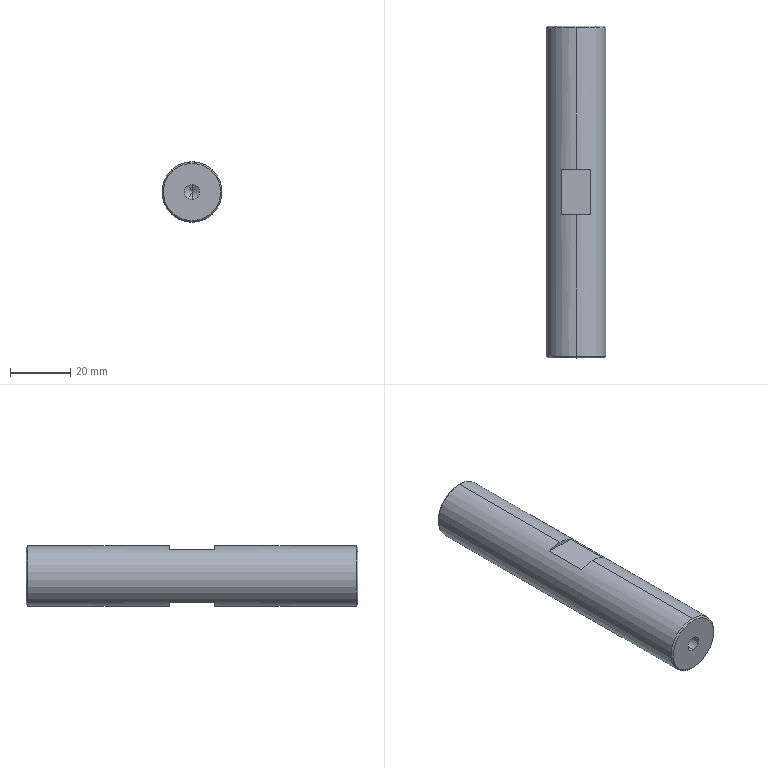Part | SolidWorks | features BaseBody 1 | 1 solid | 22 faces | box 20 x 110 x 20 mm | volume 33688 mm3 | cone 8 | plane 8 | cylinder 6 | commonest cylinder face diameters 5 x4 20 x2
STEP:
#1=CARTESIAN_POINT('',(0.,15.,2.5));
#2=VERTEX_POINT('',#1);
#3=CARTESIAN_POINT('',(0.,15.,-2.5));
#4=VERTEX_POINT('',#3);
#5=CARTESIAN_POINT('',(0.,15.,0.));
#6=DIRECTION('',(0.,-1.,0.));
#7=DIRECTION('',(0.,0.,-1.));
#8=AXIS2_PLACEMENT_3D('',#5,#6,#7);
#9=CIRCLE('',#8,2.5);
#10=EDGE_CURVE('',#2,#4,#9,.T.);
#11=ORIENTED_EDGE('',*,*,#10,.F.);
#12=CARTESIAN_POINT('',(0.,0.,2.5));
#13=VERTEX_POINT('',#12);
#14=CARTESIAN_POINT('',(0.,0.,2.5));
#15=DIRECTION('',(0.,-1.,0.));
#16=VECTOR('',#15,1000.);
#17=LINE('',#14,#16);
#18=EDGE_CURVE('',#2,#13,#17,.T.);
#19=ORIENTED_EDGE('',*,*,#18,.T.);
#20=CARTESIAN_POINT('',(0.,0.,-2.5));
#21=VERTEX_POINT('',#20);
#22=CARTESIAN_POINT('',(0.,0.,0.));
#23=DIRECTION('',(0.,-1.,0.));
#24=DIRECTION('',(0.,0.,-1.));
#25=AXIS2_PLACEMENT_3D('',#22,#23,#24);
#26=CIRCLE('',#25,2.5);
#27=EDGE_CURVE('',#13,#21,#26,.T.);
#28=ORIENTED_EDGE('',*,*,#27,.T.);
#29=CARTESIAN_POINT('',(0.,0.,-2.5));
#30=DIRECTION('',(0.,-1.,0.));
#31=VECTOR('',#30,1000.);
#32=LINE('',#29,#31);
#33=EDGE_CURVE('',#4,#21,#32,.T.);
#34=ORIENTED_EDGE('',*,*,#33,.F.);
#35=EDGE_LOOP('',(#11,#19,#28,#34));
#36=FACE_OUTER_BOUND('',#35,.T.);
#37=CARTESIAN_POINT('',(0.,0.,0.));
#38=DIRECTION('',(0.,-1.,0.));
#39=DIRECTION('',(0.,0.,-1.));
#40=AXIS2_PLACEMENT_3D('',#37,#38,#39);
#41=CYLINDRICAL_SURFACE('',#40,2.5);
#42=ADVANCED_FACE('',(#36),#41,.F.);
#43=CARTESIAN_POINT('',(0.,16.502,0.));
#44=VERTEX_POINT('',#43);
#45=CARTESIAN_POINT('',(0.,15.,-2.5));
#46=DIRECTION('',(0.,-0.515,-0.8572));
#47=VECTOR('',#46,1000.);
#48=LINE('',#45,#47);
#49=EDGE_CURVE('',#44,#4,#48,.T.);
#50=ORIENTED_EDGE('',*,*,#49,.F.);
#51=CARTESIAN_POINT('',(0.,15.,2.5));
#52=DIRECTION('',(0.,-0.515,0.8572));
#53=VECTOR('',#52,1000.);
#54=LINE('',#51,#53);
#55=EDGE_CURVE('',#44,#2,#54,.T.);
#56=ORIENTED_EDGE('',*,*,#55,.T.);
#57=ORIENTED_EDGE('',*,*,#10,.T.);
#58=EDGE_LOOP('',(#50,#56,#57));
#59=FACE_OUTER_BOUND('',#58,.T.);
#60=CARTESIAN_POINT('',(0.,15.,0.));
#61=DIRECTION('',(0.,-1.,0.));
#62=DIRECTION('',(0.,0.,-1.));
#63=AXIS2_PLACEMENT_3D('',#60,#61,#62);
#64=CONICAL_SURFACE('',#63,2.5,1.03);
#65=ADVANCED_FACE('',(#59),#64,.F.);
#66=CARTESIAN_POINT('',(0.,95.,-2.5));
#67=VERTEX_POINT('',#66);
#68=CARTESIAN_POINT('',(0.,95.,2.5));
#69=VERTEX_POINT('',#68);
#70=CARTESIAN_POINT('',(0.,95.,0.));
#71=DIRECTION('',(0.,1.,0.));
#72=DIRECTION('',(0.,0.,1.));
#73=AXIS2_PLACEMENT_3D('',#70,#71,#72);
#74=CIRCLE('',#73,2.5);
#75=EDGE_CURVE('',#67,#69,#74,.T.);
#76=ORIENTED_EDGE('',*,*,#75,.F.);
#77=CARTESIAN_POINT('',(0.,110.,-2.5));
#78=VERTEX_POINT('',#77);
#79=CARTESIAN_POINT('',(0.,110.,-2.5));
#80=DIRECTION('',(0.,1.,0.));
#81=VECTOR('',#80,1000.);
#82=LINE('',#79,#81);
#83=EDGE_CURVE('',#67,#78,#82,.T.);
#84=ORIENTED_EDGE('',*,*,#83,.T.);
#85=CARTESIAN_POINT('',(0.,110.,2.5));
#86=VERTEX_POINT('',#85);
#87=CARTESIAN_POINT('',(0.,110.,0.));
#88=DIRECTION('',(0.,1.,0.));
#89=DIRECTION('',(0.,0.,1.));
#90=AXIS2_PLACEMENT_3D('',#87,#88,#89);
#91=CIRCLE('',#90,2.5);
#92=EDGE_CURVE('',#78,#86,#91,.T.);
#93=ORIENTED_EDGE('',*,*,#92,.T.);
#94=CARTESIAN_POINT('',(0.,110.,2.5));
#95=DIRECTION('',(0.,1.,0.));
#96=VECTOR('',#95,1000.);
#97=LINE('',#94,#96);
#98=EDGE_CURVE('',#69,#86,#97,.T.);
#99=ORIENTED_EDGE('',*,*,#98,.F.);
#100=EDGE_LOOP('',(#76,#84,#93,#99));
#101=FACE_OUTER_BOUND('',#100,.T.);
#102=CARTESIAN_POINT('',(0.,110.,0.));
#103=DIRECTION('',(0.,1.,0.));
#104=DIRECTION('',(0.,0.,1.));
#105=AXIS2_PLACEMENT_3D('',#102,#103,#104);
#106=CYLINDRICAL_SURFACE('',#105,2.5);
#107=ADVANCED_FACE('',(#101),#106,.F.);
#108=CARTESIAN_POINT('',(0.,93.498,0.));
#109=VERTEX_POINT('',#108);
#110=CARTESIAN_POINT('',(0.,95.,2.5));
#111=DIRECTION('',(0.,0.515,0.8572));
#112=VECTOR('',#111,1000.);
#113=LINE('',#110,#112);
#114=EDGE_CURVE('',#109,#69,#113,.T.);
#115=ORIENTED_EDGE('',*,*,#114,.F.);
#116=CARTESIAN_POINT('',(0.,95.,-2.5));
#117=DIRECTION('',(0.,0.515,-0.8572));
#118=VECTOR('',#117,1000.);
#119=LINE('',#116,#118);
#120=EDGE_CURVE('',#109,#67,#119,.T.);
#121=ORIENTED_EDGE('',*,*,#120,.T.);
#122=ORIENTED_EDGE('',*,*,#75,.T.);
#123=EDGE_LOOP('',(#115,#121,#122));
#124=FACE_OUTER_BOUND('',#123,.T.);
#125=CARTESIAN_POINT('',(0.,95.,0.));
#126=DIRECTION('',(0.,1.,0.));
#127=DIRECTION('',(0.,0.,1.));
#128=AXIS2_PLACEMENT_3D('',#125,#126,#127);
#129=CONICAL_SURFACE('',#128,2.5,1.03);
#130=ADVANCED_FACE('',(#124),#129,.F.);
#131=CARTESIAN_POINT('',(0.,110.,9.5));
#132=VERTEX_POINT('',#131);
#133=CARTESIAN_POINT('',(0.,110.,-9.5));
#134=VERTEX_POINT('',#133);
#135=CARTESIAN_POINT('',(0.,110.,0.));
#136=DIRECTION('',(0.,1.,0.));
#137=DIRECTION('',(0.,0.,1.));
#138=AXIS2_PLACEMENT_3D('',#135,#136,#137);
#139=CIRCLE('',#138,9.5);
#140=EDGE_CURVE('',#132,#134,#139,.T.);
#141=ORIENTED_EDGE('',*,*,#140,.F.);
#142=CARTESIAN_POINT('',(0.,109.5,10.));
#143=VERTEX_POINT('',#142);
#144=CARTESIAN_POINT('',(0.,110.,9.5));
#145=DIRECTION('',(0.,-0.7071,0.7071));
#146=VECTOR('',#145,1000.);
#147=LINE('',#144,#146);
#148=EDGE_CURVE('',#132,#143,#147,.T.);
#149=ORIENTED_EDGE('',*,*,#148,.T.);
#150=CARTESIAN_POINT('',(0.,109.5,-10.));
#151=VERTEX_POINT('',#150);
#152=CARTESIAN_POINT('',(0.,109.5,0.));
#153=DIRECTION('',(0.,-1.,0.));
#154=DIRECTION('',(0.,0.,1.));
#155=AXIS2_PLACEMENT_3D('',#152,#153,#154);
#156=CIRCLE('',#155,10.);
#157=EDGE_CURVE('',#151,#143,#156,.T.);
#158=ORIENTED_EDGE('',*,*,#157,.F.);
#159=CARTESIAN_POINT('',(0.,110.,-9.5));
#160=DIRECTION('',(0.,-0.7071,-0.7071));
#161=VECTOR('',#160,1000.);
#162=LINE('',#159,#161);
#163=EDGE_CURVE('',#134,#151,#162,.T.);
#164=ORIENTED_EDGE('',*,*,#163,.F.);
#165=EDGE_LOOP('',(#141,#149,#158,#164));
#166=FACE_OUTER_BOUND('',#165,.T.);
#167=CARTESIAN_POINT('',(0.,110.,0.));
#168=DIRECTION('',(0.,-1.,0.));
#169=DIRECTION('',(0.,0.,-1.));
#170=AXIS2_PLACEMENT_3D('',#167,#168,#169);
#171=CONICAL_SURFACE('',#170,9.5,0.7854);
#172=ADVANCED_FACE('',(#166),#171,.T.);
#173=CARTESIAN_POINT('',(0.,0.,-9.5));
#174=VERTEX_POINT('',#173);
#175=CARTESIAN_POINT('',(0.,0.,9.5));
#176=VERTEX_POINT('',#175);
#177=CARTESIAN_POINT('',(0.,0.,0.));
#178=DIRECTION('',(0.,-1.,0.));
#179=DIRECTION('',(0.,0.,1.));
#180=AXIS2_PLACEMENT_3D('',#177,#178,#179);
#181=CIRCLE('',#180,9.5);
#182=EDGE_CURVE('',#174,#176,#181,.T.);
#183=ORIENTED_EDGE('',*,*,#182,.F.);
#184=CARTESIAN_POINT('',(0.,0.5,-10.));
#185=VERTEX_POINT('',#184);
#186=CARTESIAN_POINT('',(0.,0.5,-10.));
#187=DIRECTION('',(0.,0.7071,-0.7071));
#188=VECTOR('',#187,1000.);
#189=LINE('',#186,#188);
#190=EDGE_CURVE('',#174,#185,#189,.T.);
#191=ORIENTED_EDGE('',*,*,#190,.T.);
#192=CARTESIAN_POINT('',(0.,0.5,10.));
#193=VERTEX_POINT('',#192);
#194=CARTESIAN_POINT('',(0.,0.5,0.));
#195=DIRECTION('',(0.,1.,0.));
#196=DIRECTION('',(0.,0.,1.));
#197=AXIS2_PLACEMENT_3D('',#194,#195,#196);
#198=CIRCLE('',#197,10.);
#199=EDGE_CURVE('',#193,#185,#198,.T.);
#200=ORIENTED_EDGE('',*,*,#199,.F.);
#201=CARTESIAN_POINT('',(0.,0.5,10.));
#202=DIRECTION('',(0.,0.7071,0.7071));
#203=VECTOR('',#202,1000.);
#204=LINE('',#201,#203);
#205=EDGE_CURVE('',#176,#193,#204,.T.);
#206=ORIENTED_EDGE('',*,*,#205,.F.);
#207=EDGE_LOOP('',(#183,#191,#200,#206));
#208=FACE_OUTER_BOUND('',#207,.T.);
#209=CARTESIAN_POINT('',(0.,0.5,0.));
#210=DIRECTION('',(0.,1.,0.));
#211=DIRECTION('',(0.,0.,1.));
#212=AXIS2_PLACEMENT_3D('',#209,#210,#211);
#213=CONICAL_SURFACE('',#212,10.,0.7854);
#214=ADVANCED_FACE('',(#208),#213,.T.);
#215=ORIENTED_EDGE('',*,*,#157,.T.);
#216=CARTESIAN_POINT('',(0.,62.5,10.));
#217=VERTEX_POINT('',#216);
#218=CARTESIAN_POINT('',(0.,110.,10.));
#219=DIRECTION('',(0.,-1.,0.));
#220=VECTOR('',#219,1000.);
#221=LINE('',#218,#220);
#222=EDGE_CURVE('',#143,#217,#221,.T.);
#223=ORIENTED_EDGE('',*,*,#222,.T.);
#224=CARTESIAN_POINT('',(4.841,62.5,8.75));
#225=VERTEX_POINT('',#224);
#226=CARTESIAN_POINT('',(0.,62.5,0.));
#227=DIRECTION('',(0.,1.,0.));
#228=DIRECTION('',(0.,0.,1.));
#229=AXIS2_PLACEMENT_3D('',#226,#227,#228);
#230=CIRCLE('',#229,10.);
#231=EDGE_CURVE('',#217,#225,#230,.T.);
#232=ORIENTED_EDGE('',*,*,#231,.T.);
#233=CARTESIAN_POINT('',(4.841,47.5,8.75));
#234=VERTEX_POINT('',#233);
#235=CARTESIAN_POINT('',(4.841,110.,8.75));
#236=DIRECTION('',(0.,-1.,0.));
#237=VECTOR('',#236,1000.);
#238=LINE('',#235,#237);
#239=EDGE_CURVE('',#225,#234,#238,.T.);
#240=ORIENTED_EDGE('',*,*,#239,.T.);
#241=CARTESIAN_POINT('',(0.,47.5,10.));
#242=VERTEX_POINT('',#241);
#243=CARTESIAN_POINT('',(0.,47.5,0.));
#244=DIRECTION('',(0.,-1.,0.));
#245=DIRECTION('',(0.,0.,-1.));
#246=AXIS2_PLACEMENT_3D('',#243,#244,#245);
#247=CIRCLE('',#246,10.);
#248=EDGE_CURVE('',#234,#242,#247,.T.);
#249=ORIENTED_EDGE('',*,*,#248,.T.);
#250=CARTESIAN_POINT('',(0.,110.,10.));
#251=DIRECTION('',(0.,-1.,0.));
#252=VECTOR('',#251,1000.);
#253=LINE('',#250,#252);
#254=EDGE_CURVE('',#242,#193,#253,.T.);
#255=ORIENTED_EDGE('',*,*,#254,.T.);
#256=ORIENTED_EDGE('',*,*,#199,.T.);
#257=CARTESIAN_POINT('',(0.,47.5,-10.));
#258=VERTEX_POINT('',#257);
#259=CARTESIAN_POINT('',(0.,110.,-10.));
#260=DIRECTION('',(0.,-1.,0.));
#261=VECTOR('',#260,1000.);
#262=LINE('',#259,#261);
#263=EDGE_CURVE('',#258,#185,#262,.T.);
#264=ORIENTED_EDGE('',*,*,#263,.F.);
#265=CARTESIAN_POINT('',(4.841,47.5,-8.75));
#266=VERTEX_POINT('',#265);
#267=CARTESIAN_POINT('',(0.,47.5,0.));
#268=DIRECTION('',(0.,-1.,0.));
#269=DIRECTION('',(0.,0.,-1.));
#270=AXIS2_PLACEMENT_3D('',#267,#268,#269);
#271=CIRCLE('',#270,10.);
#272=EDGE_CURVE('',#258,#266,#271,.T.);
#273=ORIENTED_EDGE('',*,*,#272,.T.);
#274=CARTESIAN_POINT('',(4.841,62.5,-8.75));
#275=VERTEX_POINT('',#274);
#276=CARTESIAN_POINT('',(4.841,110.,-8.75));
#277=DIRECTION('',(0.,1.,0.));
#278=VECTOR('',#277,1000.);
#279=LINE('',#276,#278);
#280=EDGE_CURVE('',#266,#275,#279,.T.);
#281=ORIENTED_EDGE('',*,*,#280,.T.);
#282=CARTESIAN_POINT('',(0.,62.5,-10.));
#283=VERTEX_POINT('',#282);
#284=CARTESIAN_POINT('',(0.,62.5,0.));
#285=DIRECTION('',(0.,1.,0.));
#286=DIRECTION('',(0.,0.,1.));
#287=AXIS2_PLACEMENT_3D('',#284,#285,#286);
#288=CIRCLE('',#287,10.);
#289=EDGE_CURVE('',#275,#283,#288,.T.);
#290=ORIENTED_EDGE('',*,*,#289,.T.);
#291=CARTESIAN_POINT('',(0.,110.,-10.));
#292=DIRECTION('',(0.,-1.,0.));
#293=VECTOR('',#292,1000.);
#294=LINE('',#291,#293);
#295=EDGE_CURVE('',#151,#283,#294,.T.);
#296=ORIENTED_EDGE('',*,*,#295,.F.);
#297=EDGE_LOOP('',(#215,#223,#232,#240,#249,#255,#256,#264,#273,#281,#290,#296));
#298=FACE_OUTER_BOUND('',#297,.T.);
#299=CARTESIAN_POINT('',(0.,110.,0.));
#300=DIRECTION('',(0.,-1.,0.));
#301=DIRECTION('',(0.,0.,-1.));
#302=AXIS2_PLACEMENT_3D('',#299,#300,#301);
#303=CYLINDRICAL_SURFACE('',#302,10.);
#304=ADVANCED_FACE('',(#298),#303,.T.);
#305=CARTESIAN_POINT('',(-4.841,62.5,-8.75));
#306=VERTEX_POINT('',#305);
#307=CARTESIAN_POINT('',(-10.,62.5,-8.75));
#308=DIRECTION('',(1.,0.,0.));
#309=VECTOR('',#308,1000.);
#310=LINE('',#307,#309);
#311=EDGE_CURVE('',#306,#275,#310,.T.);
#312=ORIENTED_EDGE('',*,*,#311,.F.);
#313=CARTESIAN_POINT('',(0.,62.5,0.));
#314=DIRECTION('',(0.,1.,0.));
#315=DIRECTION('',(0.,0.,1.));
#316=AXIS2_PLACEMENT_3D('',#313,#314,#315);
#317=CIRCLE('',#316,10.);
#318=EDGE_CURVE('',#283,#306,#317,.T.);
#319=ORIENTED_EDGE('',*,*,#318,.F.);
#320=ORIENTED_EDGE('',*,*,#289,.F.);
#321=EDGE_LOOP('',(#312,#319,#320));
#322=FACE_OUTER_BOUND('',#321,.T.);
#323=CARTESIAN_POINT('',(-10.,62.5,-8.75));
#324=DIRECTION('',(0.,1.,0.));
#325=DIRECTION('',(1.,0.,0.));
#326=AXIS2_PLACEMENT_3D('',#323,#324,#325);
#327=PLANE('',#326);
#328=ADVANCED_FACE('',(#322),#327,.F.);
#329=ORIENTED_EDGE('',*,*,#311,.T.);
#330=ORIENTED_EDGE('',*,*,#280,.F.);
#331=CARTESIAN_POINT('',(-4.841,47.5,-8.75));
#332=VERTEX_POINT('',#331);
#333=CARTESIAN_POINT('',(-10.,47.5,-8.75));
#334=DIRECTION('',(1.,0.,0.));
#335=VECTOR('',#334,1000.);
#336=LINE('',#333,#335);
#337=EDGE_CURVE('',#332,#266,#336,.T.);
#338=ORIENTED_EDGE('',*,*,#337,.F.);
#339=CARTESIAN_POINT('',(-4.841,110.,-8.75));
#340=DIRECTION('',(0.,-1.,0.));
#341=VECTOR('',#340,1000.);
#342=LINE('',#339,#341);
#343=EDGE_CURVE('',#306,#332,#342,.T.);
#344=ORIENTED_EDGE('',*,*,#343,.F.);
#345=EDGE_LOOP('',(#329,#330,#338,#344));
#346=FACE_OUTER_BOUND('',#345,.T.);
#347=CARTESIAN_POINT('',(-10.,47.5,-8.75));
#348=DIRECTION('',(0.,0.,1.));
#349=DIRECTION('',(0.,-1.,0.));
#350=AXIS2_PLACEMENT_3D('',#347,#348,#349);
#351=PLANE('',#350);
#352=ADVANCED_FACE('',(#346),#351,.F.);
#353=ORIENTED_EDGE('',*,*,#337,.T.);
#354=ORIENTED_EDGE('',*,*,#272,.F.);
#355=CARTESIAN_POINT('',(0.,47.5,0.));
#356=DIRECTION('',(0.,-1.,0.));
#357=DIRECTION('',(0.,0.,-1.));
#358=AXIS2_PLACEMENT_3D('',#355,#356,#357);
#359=CIRCLE('',#358,10.);
#360=EDGE_CURVE('',#332,#258,#359,.T.);
#361=ORIENTED_EDGE('',*,*,#360,.F.);
#362=EDGE_LOOP('',(#353,#354,#361));
#363=FACE_OUTER_BOUND('',#362,.T.);
#364=CARTESIAN_POINT('',(-10.,47.5,-8.75));
#365=DIRECTION('',(0.,-1.,0.));
#366=DIRECTION('',(0.,0.,-1.));
#367=AXIS2_PLACEMENT_3D('',#364,#365,#366);
#368=PLANE('',#367);
#369=ADVANCED_FACE('',(#363),#368,.F.);
#370=CARTESIAN_POINT('',(-4.841,62.5,8.75));
#371=VERTEX_POINT('',#370);
#372=CARTESIAN_POINT('',(-10.,62.5,8.75));
#373=DIRECTION('',(1.,0.,0.));
#374=VECTOR('',#373,1000.);
#375=LINE('',#372,#374);
#376=EDGE_CURVE('',#371,#225,#375,.T.);
#377=ORIENTED_EDGE('',*,*,#376,.T.);
#378=ORIENTED_EDGE('',*,*,#231,.F.);
#379=CARTESIAN_POINT('',(0.,62.5,0.));
#380=DIRECTION('',(0.,1.,0.));
#381=DIRECTION('',(0.,0.,1.));
#382=AXIS2_PLACEMENT_3D('',#379,#380,#381);
#383=CIRCLE('',#382,10.);
#384=EDGE_CURVE('',#371,#217,#383,.T.);
#385=ORIENTED_EDGE('',*,*,#384,.F.);
#386=EDGE_LOOP('',(#377,#378,#385));
#387=FACE_OUTER_BOUND('',#386,.T.);
#388=CARTESIAN_POINT('',(-10.,62.5,11.25));
#389=DIRECTION('',(0.,1.,0.));
#390=DIRECTION('',(1.,0.,0.));
#391=AXIS2_PLACEMENT_3D('',#388,#389,#390);
#392=PLANE('',#391);
#393=ADVANCED_FACE('',(#387),#392,.F.);
#394=CARTESIAN_POINT('',(-4.841,47.5,8.75));
#395=VERTEX_POINT('',#394);
#396=CARTESIAN_POINT('',(-10.,47.5,8.75));
#397=DIRECTION('',(1.,0.,0.));
#398=VECTOR('',#397,1000.);
#399=LINE('',#396,#398);
#400=EDGE_CURVE('',#395,#234,#399,.T.);
#401=ORIENTED_EDGE('',*,*,#400,.F.);
#402=CARTESIAN_POINT('',(0.,47.5,0.));
#403=DIRECTION('',(0.,-1.,0.));
#404=DIRECTION('',(0.,0.,-1.));
#405=AXIS2_PLACEMENT_3D('',#402,#403,#404);
#406=CIRCLE('',#405,10.);
#407=EDGE_CURVE('',#242,#395,#406,.T.);
#408=ORIENTED_EDGE('',*,*,#407,.F.);
#409=ORIENTED_EDGE('',*,*,#248,.F.);
#410=EDGE_LOOP('',(#401,#408,#409));
#411=FACE_OUTER_BOUND('',#410,.T.);
#412=CARTESIAN_POINT('',(-10.,47.5,11.25));
#413=DIRECTION('',(0.,-1.,0.));
#414=DIRECTION('',(0.,0.,-1.));
#415=AXIS2_PLACEMENT_3D('',#412,#413,#414);
#416=PLANE('',#415);
#417=ADVANCED_FACE('',(#411),#416,.F.);
#418=ORIENTED_EDGE('',*,*,#376,.F.);
#419=CARTESIAN_POINT('',(-4.841,110.,8.75));
#420=DIRECTION('',(0.,1.,0.));
#421=VECTOR('',#420,1000.);
#422=LINE('',#419,#421);
#423=EDGE_CURVE('',#395,#371,#422,.T.);
#424=ORIENTED_EDGE('',*,*,#423,.F.);
#425=ORIENTED_EDGE('',*,*,#400,.T.);
#426=ORIENTED_EDGE('',*,*,#239,.F.);
#427=EDGE_LOOP('',(#418,#424,#425,#426));
#428=FACE_OUTER_BOUND('',#427,.T.);
#429=CARTESIAN_POINT('',(-10.,47.5,8.75));
#430=DIRECTION('',(0.,0.,-1.));
#431=DIRECTION('',(0.,-1.,0.));
#432=AXIS2_PLACEMENT_3D('',#429,#430,#431);
#433=PLANE('',#432);
#434=ADVANCED_FACE('',(#428),#433,.F.);
#435=CARTESIAN_POINT('',(0.,0.,0.));
#436=DIRECTION('',(0.,-1.,0.));
#437=DIRECTION('',(0.,0.,-1.));
#438=AXIS2_PLACEMENT_3D('',#435,#436,#437);
#439=CIRCLE('',#438,2.5);
#440=EDGE_CURVE('',#21,#13,#439,.T.);
#441=ORIENTED_EDGE('',*,*,#440,.F.);
#442=ORIENTED_EDGE('',*,*,#27,.F.);
#443=EDGE_LOOP('',(#441,#442));
#444=FACE_BOUND('',#443,.T.);
#445=CARTESIAN_POINT('',(0.,0.,0.));
#446=DIRECTION('',(0.,-1.,0.));
#447=DIRECTION('',(0.,0.,1.));
#448=AXIS2_PLACEMENT_3D('',#445,#446,#447);
#449=CIRCLE('',#448,9.5);
#450=EDGE_CURVE('',#176,#174,#449,.T.);
#451=ORIENTED_EDGE('',*,*,#450,.T.);
#452=ORIENTED_EDGE('',*,*,#182,.T.);
#453=EDGE_LOOP('',(#451,#452));
#454=FACE_OUTER_BOUND('',#453,.T.);
#455=CARTESIAN_POINT('',(0.,0.,0.));
#456=DIRECTION('',(0.,1.,0.));
#457=DIRECTION('',(1.,0.,0.));
#458=AXIS2_PLACEMENT_3D('',#455,#456,#457);
#459=PLANE('',#458);
#460=ADVANCED_FACE('',(#444,#454),#459,.F.);
#461=CARTESIAN_POINT('',(0.,110.,0.));
#462=DIRECTION('',(0.,1.,0.));
#463=DIRECTION('',(0.,0.,1.));
#464=AXIS2_PLACEMENT_3D('',#461,#462,#463);
#465=CIRCLE('',#464,2.5);
#466=EDGE_CURVE('',#86,#78,#465,.T.);
#467=ORIENTED_EDGE('',*,*,#466,.F.);
#468=ORIENTED_EDGE('',*,*,#92,.F.);
#469=EDGE_LOOP('',(#467,#468));
#470=FACE_BOUND('',#469,.T.);
#471=CARTESIAN_POINT('',(0.,110.,0.));
#472=DIRECTION('',(0.,1.,0.));
#473=DIRECTION('',(0.,0.,1.));
#474=AXIS2_PLACEMENT_3D('',#471,#472,#473);
#475=CIRCLE('',#474,9.5);
#476=EDGE_CURVE('',#134,#132,#475,.T.);
#477=ORIENTED_EDGE('',*,*,#476,.T.);
#478=ORIENTED_EDGE('',*,*,#140,.T.);
#479=EDGE_LOOP('',(#477,#478));
#480=FACE_OUTER_BOUND('',#479,.T.);
#481=CARTESIAN_POINT('',(0.,110.,0.));
#482=DIRECTION('',(0.,1.,0.));
#483=DIRECTION('',(1.,0.,0.));
#484=AXIS2_PLACEMENT_3D('',#481,#482,#483);
#485=PLANE('',#484);
#486=ADVANCED_FACE('',(#470,#480),#485,.T.);
#487=ORIENTED_EDGE('',*,*,#222,.F.);
#488=CARTESIAN_POINT('',(0.,109.5,0.));
#489=DIRECTION('',(0.,-1.,0.));
#490=DIRECTION('',(0.,0.,1.));
#491=AXIS2_PLACEMENT_3D('',#488,#489,#490);
#492=CIRCLE('',#491,10.);
#493=EDGE_CURVE('',#143,#151,#492,.T.);
#494=ORIENTED_EDGE('',*,*,#493,.T.);
#495=ORIENTED_EDGE('',*,*,#295,.T.);
#496=ORIENTED_EDGE('',*,*,#318,.T.);
#497=ORIENTED_EDGE('',*,*,#343,.T.);
#498=ORIENTED_EDGE('',*,*,#360,.T.);
#499=ORIENTED_EDGE('',*,*,#263,.T.);
#500=CARTESIAN_POINT('',(0.,0.5,0.));
#501=DIRECTION('',(0.,1.,0.));
#502=DIRECTION('',(0.,0.,1.));
#503=AXIS2_PLACEMENT_3D('',#500,#501,#502);
#504=CIRCLE('',#503,10.);
#505=EDGE_CURVE('',#185,#193,#504,.T.);
#506=ORIENTED_EDGE('',*,*,#505,.T.);
#507=ORIENTED_EDGE('',*,*,#254,.F.);
#508=ORIENTED_EDGE('',*,*,#407,.T.);
#509=ORIENTED_EDGE('',*,*,#423,.T.);
#510=ORIENTED_EDGE('',*,*,#384,.T.);
#511=EDGE_LOOP('',(#487,#494,#495,#496,#497,#498,#499,#506,#507,#508,#509,#510));
#512=FACE_OUTER_BOUND('',#511,.T.);
#513=CARTESIAN_POINT('',(0.,110.,0.));
#514=DIRECTION('',(0.,-1.,0.));
#515=DIRECTION('',(0.,0.,-1.));
#516=AXIS2_PLACEMENT_3D('',#513,#514,#515);
#517=CYLINDRICAL_SURFACE('',#516,10.);
#518=ADVANCED_FACE('',(#512),#517,.T.);
#519=ORIENTED_EDGE('',*,*,#190,.F.);
#520=ORIENTED_EDGE('',*,*,#450,.F.);
#521=ORIENTED_EDGE('',*,*,#205,.T.);
#522=ORIENTED_EDGE('',*,*,#505,.F.);
#523=EDGE_LOOP('',(#519,#520,#521,#522));
#524=FACE_OUTER_BOUND('',#523,.T.);
#525=CARTESIAN_POINT('',(0.,0.5,0.));
#526=DIRECTION('',(0.,1.,0.));
#527=DIRECTION('',(0.,0.,1.));
#528=AXIS2_PLACEMENT_3D('',#525,#526,#527);
#529=CONICAL_SURFACE('',#528,10.,0.7854);
#530=ADVANCED_FACE('',(#524),#529,.T.);
#531=ORIENTED_EDGE('',*,*,#148,.F.);
#532=ORIENTED_EDGE('',*,*,#476,.F.);
#533=ORIENTED_EDGE('',*,*,#163,.T.);
#534=ORIENTED_EDGE('',*,*,#493,.F.);
#535=EDGE_LOOP('',(#531,#532,#533,#534));
#536=FACE_OUTER_BOUND('',#535,.T.);
#537=CARTESIAN_POINT('',(0.,110.,0.));
#538=DIRECTION('',(0.,-1.,0.));
#539=DIRECTION('',(0.,0.,-1.));
#540=AXIS2_PLACEMENT_3D('',#537,#538,#539);
#541=CONICAL_SURFACE('',#540,9.5,0.7854);
#542=ADVANCED_FACE('',(#536),#541,.T.);
#543=ORIENTED_EDGE('',*,*,#120,.F.);
#544=ORIENTED_EDGE('',*,*,#114,.T.);
#545=CARTESIAN_POINT('',(0.,95.,0.));
#546=DIRECTION('',(0.,1.,0.));
#547=DIRECTION('',(0.,0.,1.));
#548=AXIS2_PLACEMENT_3D('',#545,#546,#547);
#549=CIRCLE('',#548,2.5);
#550=EDGE_CURVE('',#69,#67,#549,.T.);
#551=ORIENTED_EDGE('',*,*,#550,.T.);
#552=EDGE_LOOP('',(#543,#544,#551));
#553=FACE_OUTER_BOUND('',#552,.T.);
#554=CARTESIAN_POINT('',(0.,95.,0.));
#555=DIRECTION('',(0.,1.,0.));
#556=DIRECTION('',(0.,0.,1.));
#557=AXIS2_PLACEMENT_3D('',#554,#555,#556);
#558=CONICAL_SURFACE('',#557,2.5,1.03);
#559=ADVANCED_FACE('',(#553),#558,.F.);
#560=ORIENTED_EDGE('',*,*,#83,.F.);
#561=ORIENTED_EDGE('',*,*,#550,.F.);
#562=ORIENTED_EDGE('',*,*,#98,.T.);
#563=ORIENTED_EDGE('',*,*,#466,.T.);
#564=EDGE_LOOP('',(#560,#561,#562,#563));
#565=FACE_OUTER_BOUND('',#564,.T.);
#566=CARTESIAN_POINT('',(0.,110.,0.));
#567=DIRECTION('',(0.,1.,0.));
#568=DIRECTION('',(0.,0.,1.));
#569=AXIS2_PLACEMENT_3D('',#566,#567,#568);
#570=CYLINDRICAL_SURFACE('',#569,2.5);
#571=ADVANCED_FACE('',(#565),#570,.F.);
#572=ORIENTED_EDGE('',*,*,#55,.F.);
#573=ORIENTED_EDGE('',*,*,#49,.T.);
#574=CARTESIAN_POINT('',(0.,15.,0.));
#575=DIRECTION('',(0.,-1.,0.));
#576=DIRECTION('',(0.,0.,-1.));
#577=AXIS2_PLACEMENT_3D('',#574,#575,#576);
#578=CIRCLE('',#577,2.5);
#579=EDGE_CURVE('',#4,#2,#578,.T.);
#580=ORIENTED_EDGE('',*,*,#579,.T.);
#581=EDGE_LOOP('',(#572,#573,#580));
#582=FACE_OUTER_BOUND('',#581,.T.);
#583=CARTESIAN_POINT('',(0.,15.,0.));
#584=DIRECTION('',(0.,-1.,0.));
#585=DIRECTION('',(0.,0.,-1.));
#586=AXIS2_PLACEMENT_3D('',#583,#584,#585);
#587=CONICAL_SURFACE('',#586,2.5,1.03);
#588=ADVANCED_FACE('',(#582),#587,.F.);
#589=ORIENTED_EDGE('',*,*,#18,.F.);
#590=ORIENTED_EDGE('',*,*,#579,.F.);
#591=ORIENTED_EDGE('',*,*,#33,.T.);
#592=ORIENTED_EDGE('',*,*,#440,.T.);
#593=EDGE_LOOP('',(#589,#590,#591,#592));
#594=FACE_OUTER_BOUND('',#593,.T.);
#595=CARTESIAN_POINT('',(0.,0.,0.));
#596=DIRECTION('',(0.,-1.,0.));
#597=DIRECTION('',(0.,0.,-1.));
#598=AXIS2_PLACEMENT_3D('',#595,#596,#597);
#599=CYLINDRICAL_SURFACE('',#598,2.5);
#600=ADVANCED_FACE('',(#594),#599,.F.);
#601=CLOSED_SHELL('',(#42,#65,#107,#130,#172,#214,#304,#328,#352,#369,#393,#417,#434,#460,#486,#518,#530,#542,#559,#571,#588,#600));
#602=MANIFOLD_SOLID_BREP('',#601);
#603=CARTESIAN_POINT('',(0.,0.,0.));
#604=DIRECTION('',(0.,0.,1.));
#605=DIRECTION('',(1.,0.,0.));
#606=AXIS2_PLACEMENT_3D('',#603,#604,#605);
#607=(LENGTH_UNIT()NAMED_UNIT(*)SI_UNIT(.MILLI.,.METRE.));
#608=UNCERTAINTY_MEASURE_WITH_UNIT(LENGTH_MEASURE(0.00001),#607,'','');
#609=(NAMED_UNIT(*)PLANE_ANGLE_UNIT()SI_UNIT($,.RADIAN.));
#610=(NAMED_UNIT(*)SI_UNIT($,.STERADIAN.)SOLID_ANGLE_UNIT());
#611=(GEOMETRIC_REPRESENTATION_CONTEXT(3)GLOBAL_UNCERTAINTY_ASSIGNED_CONTEXT((#608))GLOBAL_UNIT_ASSIGNED_CONTEXT((#607,#609,#610))REPRESENTATION_CONTEXT('',''));
#612=ADVANCED_BREP_SHAPE_REPRESENTATION('',(#602,#606),#611);